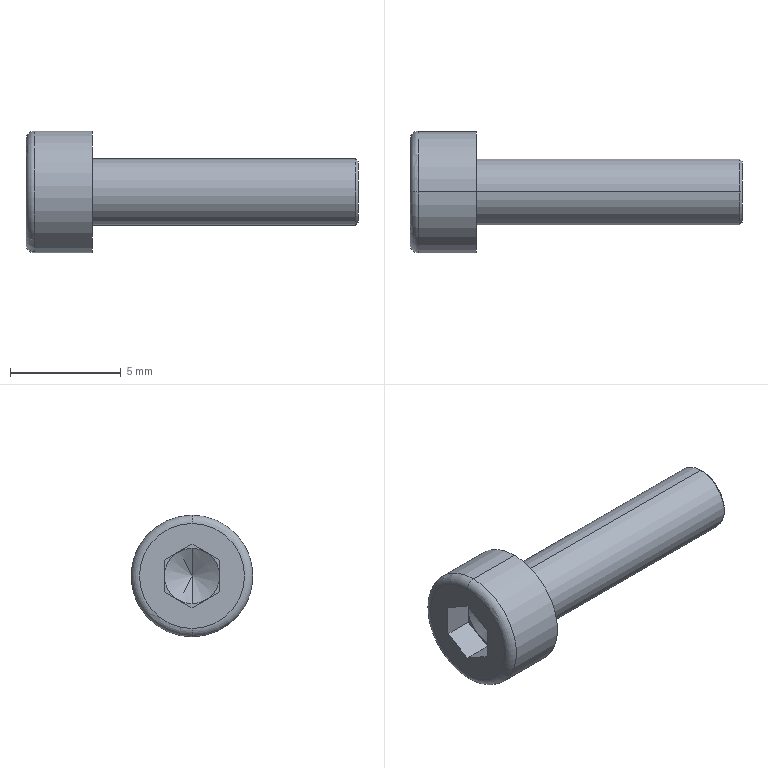Part | SolidWorks | features Fillet 2, RevCut 2, Boss 1, Chamfer 1, Cut 1, Extrusion 1, LPattern 1 | 1 solid | 25 faces | box 15 x 5.5 x 5.5 mm | volume 147.329 mm3 | plane 15 | cone 4 | cylinder 4 | torus 2 | commonest cylinder face diameters 3 x2 5.5 x2
STEP:
#1=CARTESIAN_POINT('',(15.,0.,-1.4));
#2=VERTEX_POINT('',#1);
#3=CARTESIAN_POINT('',(15.,0.,1.4));
#4=VERTEX_POINT('',#3);
#5=CARTESIAN_POINT('',(15.,0.,0.));
#6=DIRECTION('',(1.,0.,0.));
#7=DIRECTION('',(0.,0.,-1.));
#8=AXIS2_PLACEMENT_3D('',#5,#6,#7);
#9=CIRCLE('',#8,1.4);
#10=EDGE_CURVE('',#2,#4,#9,.T.);
#11=ORIENTED_EDGE('',*,*,#10,.F.);
#12=CARTESIAN_POINT('',(14.9,0.,-1.5));
#13=VERTEX_POINT('',#12);
#14=CARTESIAN_POINT('',(15.,0.,-1.4));
#15=DIRECTION('',(-0.7071,0.,-0.7071));
#16=VECTOR('',#15,1000.);
#17=LINE('',#14,#16);
#18=EDGE_CURVE('',#2,#13,#17,.T.);
#19=ORIENTED_EDGE('',*,*,#18,.T.);
#20=CARTESIAN_POINT('',(14.9,0.,1.5));
#21=VERTEX_POINT('',#20);
#22=CARTESIAN_POINT('',(14.9,0.,0.));
#23=DIRECTION('',(-1.,0.,0.));
#24=DIRECTION('',(0.,0.,-1.));
#25=AXIS2_PLACEMENT_3D('',#22,#23,#24);
#26=CIRCLE('',#25,1.5);
#27=EDGE_CURVE('',#21,#13,#26,.T.);
#28=ORIENTED_EDGE('',*,*,#27,.F.);
#29=CARTESIAN_POINT('',(15.,0.,1.4));
#30=DIRECTION('',(-0.7071,0.,0.7071));
#31=VECTOR('',#30,1000.);
#32=LINE('',#29,#31);
#33=EDGE_CURVE('',#4,#21,#32,.T.);
#34=ORIENTED_EDGE('',*,*,#33,.F.);
#35=EDGE_LOOP('',(#11,#19,#28,#34));
#36=FACE_OUTER_BOUND('',#35,.T.);
#37=CARTESIAN_POINT('',(15.,0.,0.));
#38=DIRECTION('',(-1.,0.,0.));
#39=DIRECTION('',(0.,0.,1.));
#40=AXIS2_PLACEMENT_3D('',#37,#38,#39);
#41=CONICAL_SURFACE('',#40,1.4,0.7854);
#42=ADVANCED_FACE('',(#36),#41,.T.);
#43=CARTESIAN_POINT('',(0.,0.,2.375));
#44=VERTEX_POINT('',#43);
#45=CARTESIAN_POINT('',(0.,0.,-2.375));
#46=VERTEX_POINT('',#45);
#47=CARTESIAN_POINT('',(0.,0.,0.));
#48=DIRECTION('',(-1.,0.,0.));
#49=DIRECTION('',(0.,0.,-1.));
#50=AXIS2_PLACEMENT_3D('',#47,#48,#49);
#51=CIRCLE('',#50,2.375);
#52=EDGE_CURVE('',#44,#46,#51,.T.);
#53=ORIENTED_EDGE('',*,*,#52,.F.);
#54=CARTESIAN_POINT('',(0.375,0.,2.75));
#55=VERTEX_POINT('',#54);
#56=CARTESIAN_POINT('',(0.375,0.,2.375));
#57=DIRECTION('',(0.,1.,0.));
#58=DIRECTION('',(0.,0.,1.));
#59=AXIS2_PLACEMENT_3D('',#56,#57,#58);
#60=CIRCLE('',#59,0.375);
#61=EDGE_CURVE('',#44,#55,#60,.T.);
#62=ORIENTED_EDGE('',*,*,#61,.T.);
#63=CARTESIAN_POINT('',(0.375,0.,-2.75));
#64=VERTEX_POINT('',#63);
#65=CARTESIAN_POINT('',(0.375,0.,0.));
#66=DIRECTION('',(1.,0.,0.));
#67=DIRECTION('',(0.,0.,-1.));
#68=AXIS2_PLACEMENT_3D('',#65,#66,#67);
#69=CIRCLE('',#68,2.75);
#70=EDGE_CURVE('',#64,#55,#69,.T.);
#71=ORIENTED_EDGE('',*,*,#70,.F.);
#72=CARTESIAN_POINT('',(0.375,0.,-2.375));
#73=DIRECTION('',(0.,-1.,0.));
#74=DIRECTION('',(0.,0.,-1.));
#75=AXIS2_PLACEMENT_3D('',#72,#73,#74);
#76=CIRCLE('',#75,0.375);
#77=EDGE_CURVE('',#46,#64,#76,.T.);
#78=ORIENTED_EDGE('',*,*,#77,.F.);
#79=EDGE_LOOP('',(#53,#62,#71,#78));
#80=FACE_OUTER_BOUND('',#79,.T.);
#81=CARTESIAN_POINT('',(0.375,0.,0.));
#82=DIRECTION('',(1.,0.,0.));
#83=DIRECTION('',(0.,0.,-1.));
#84=AXIS2_PLACEMENT_3D('',#81,#82,#83);
#85=TOROIDAL_SURFACE('',#84,2.375,0.375);
#86=ADVANCED_FACE('',(#80),#85,.T.);
#87=CARTESIAN_POINT('',(2.022,0.,0.));
#88=VERTEX_POINT('',#87);
#89=CARTESIAN_POINT('',(1.3,0.,1.25));
#90=VERTEX_POINT('',#89);
#91=CARTESIAN_POINT('',(1.3,0.,1.25));
#92=DIRECTION('',(-0.5,0.,0.866));
#93=VECTOR('',#92,1000.);
#94=LINE('',#91,#93);
#95=EDGE_CURVE('',#88,#90,#94,.T.);
#96=ORIENTED_EDGE('',*,*,#95,.F.);
#97=CARTESIAN_POINT('',(1.3,0.,-1.25));
#98=VERTEX_POINT('',#97);
#99=CARTESIAN_POINT('',(1.3,0.,-1.25));
#100=DIRECTION('',(-0.5,0.,-0.866));
#101=VECTOR('',#100,1000.);
#102=LINE('',#99,#101);
#103=EDGE_CURVE('',#88,#98,#102,.T.);
#104=ORIENTED_EDGE('',*,*,#103,.T.);
#105=CARTESIAN_POINT('',(1.3,-0.625,-1.083));
#106=VERTEX_POINT('',#105);
#107=CARTESIAN_POINT('',(1.3,0.,0.));
#108=DIRECTION('',(1.,0.,0.));
#109=DIRECTION('',(0.,0.,1.));
#110=AXIS2_PLACEMENT_3D('',#107,#108,#109);
#111=CIRCLE('',#110,1.25);
#112=EDGE_CURVE('',#106,#98,#111,.T.);
#113=ORIENTED_EDGE('',*,*,#112,.F.);
#114=CARTESIAN_POINT('',(1.3,-1.25,0.));
#115=VERTEX_POINT('',#114);
#116=CARTESIAN_POINT('',(1.3,0.,0.));
#117=DIRECTION('',(1.,0.,0.));
#118=DIRECTION('',(0.,0.,1.));
#119=AXIS2_PLACEMENT_3D('',#116,#117,#118);
#120=CIRCLE('',#119,1.25);
#121=EDGE_CURVE('',#115,#106,#120,.T.);
#122=ORIENTED_EDGE('',*,*,#121,.F.);
#123=CARTESIAN_POINT('',(1.3,-0.625,1.083));
#124=VERTEX_POINT('',#123);
#125=CARTESIAN_POINT('',(1.3,0.,0.));
#126=DIRECTION('',(1.,0.,0.));
#127=DIRECTION('',(0.,0.,1.));
#128=AXIS2_PLACEMENT_3D('',#125,#126,#127);
#129=CIRCLE('',#128,1.25);
#130=EDGE_CURVE('',#124,#115,#129,.T.);
#131=ORIENTED_EDGE('',*,*,#130,.F.);
#132=CARTESIAN_POINT('',(1.3,0.,0.));
#133=DIRECTION('',(1.,0.,0.));
#134=DIRECTION('',(0.,0.,1.));
#135=AXIS2_PLACEMENT_3D('',#132,#133,#134);
#136=CIRCLE('',#135,1.25);
#137=EDGE_CURVE('',#90,#124,#136,.T.);
#138=ORIENTED_EDGE('',*,*,#137,.F.);
#139=EDGE_LOOP('',(#96,#104,#113,#122,#131,#138));
#140=FACE_OUTER_BOUND('',#139,.T.);
#141=CARTESIAN_POINT('',(1.3,0.,0.));
#142=DIRECTION('',(-1.,0.,0.));
#143=DIRECTION('',(0.,0.,1.));
#144=AXIS2_PLACEMENT_3D('',#141,#142,#143);
#145=CONICAL_SURFACE('',#144,1.25,1.047);
#146=ADVANCED_FACE('',(#140),#145,.F.);
#147=ORIENTED_EDGE('',*,*,#27,.T.);
#148=CARTESIAN_POINT('',(3.,0.,-1.5));
#149=VERTEX_POINT('',#148);
#150=CARTESIAN_POINT('',(15.,0.,-1.5));
#151=DIRECTION('',(-1.,0.,0.));
#152=VECTOR('',#151,1000.);
#153=LINE('',#150,#152);
#154=EDGE_CURVE('',#13,#149,#153,.T.);
#155=ORIENTED_EDGE('',*,*,#154,.T.);
#156=CARTESIAN_POINT('',(3.,0.,1.5));
#157=VERTEX_POINT('',#156);
#158=CARTESIAN_POINT('',(3.,0.,0.));
#159=DIRECTION('',(1.,0.,0.));
#160=DIRECTION('',(0.,0.,-1.));
#161=AXIS2_PLACEMENT_3D('',#158,#159,#160);
#162=CIRCLE('',#161,1.5);
#163=EDGE_CURVE('',#149,#157,#162,.T.);
#164=ORIENTED_EDGE('',*,*,#163,.T.);
#165=CARTESIAN_POINT('',(15.,0.,1.5));
#166=DIRECTION('',(-1.,0.,0.));
#167=VECTOR('',#166,1000.);
#168=LINE('',#165,#167);
#169=EDGE_CURVE('',#21,#157,#168,.T.);
#170=ORIENTED_EDGE('',*,*,#169,.F.);
#171=EDGE_LOOP('',(#147,#155,#164,#170));
#172=FACE_OUTER_BOUND('',#171,.T.);
#173=CARTESIAN_POINT('',(15.,0.,0.));
#174=DIRECTION('',(-1.,0.,0.));
#175=DIRECTION('',(0.,0.,1.));
#176=AXIS2_PLACEMENT_3D('',#173,#174,#175);
#177=CYLINDRICAL_SURFACE('',#176,1.5);
#178=ADVANCED_FACE('',(#172),#177,.T.);
#179=CARTESIAN_POINT('',(3.,0.,-2.75));
#180=VERTEX_POINT('',#179);
#181=CARTESIAN_POINT('',(3.,0.,2.75));
#182=VERTEX_POINT('',#181);
#183=CARTESIAN_POINT('',(3.,0.,0.));
#184=DIRECTION('',(1.,0.,0.));
#185=DIRECTION('',(0.,0.,-1.));
#186=AXIS2_PLACEMENT_3D('',#183,#184,#185);
#187=CIRCLE('',#186,2.75);
#188=EDGE_CURVE('',#180,#182,#187,.T.);
#189=ORIENTED_EDGE('',*,*,#188,.F.);
#190=CARTESIAN_POINT('',(3.,0.,-2.75));
#191=DIRECTION('',(-1.,0.,0.));
#192=VECTOR('',#191,1000.);
#193=LINE('',#190,#192);
#194=EDGE_CURVE('',#180,#64,#193,.T.);
#195=ORIENTED_EDGE('',*,*,#194,.T.);
#196=ORIENTED_EDGE('',*,*,#70,.T.);
#197=CARTESIAN_POINT('',(3.,0.,2.75));
#198=DIRECTION('',(-1.,0.,0.));
#199=VECTOR('',#198,1000.);
#200=LINE('',#197,#199);
#201=EDGE_CURVE('',#182,#55,#200,.T.);
#202=ORIENTED_EDGE('',*,*,#201,.F.);
#203=EDGE_LOOP('',(#189,#195,#196,#202));
#204=FACE_OUTER_BOUND('',#203,.T.);
#205=CARTESIAN_POINT('',(3.,0.,0.));
#206=DIRECTION('',(-1.,0.,0.));
#207=DIRECTION('',(0.,0.,1.));
#208=AXIS2_PLACEMENT_3D('',#205,#206,#207);
#209=CYLINDRICAL_SURFACE('',#208,2.75);
#210=ADVANCED_FACE('',(#204),#209,.T.);
#211=CARTESIAN_POINT('',(1.3,-1.25,0.7217));
#212=VERTEX_POINT('',#211);
#213=CARTESIAN_POINT('',(1.3,0.,1.443));
#214=DIRECTION('',(0.,-0.866,-0.5));
#215=VECTOR('',#214,1000.);
#216=LINE('',#213,#215);
#217=EDGE_CURVE('',#124,#212,#216,.T.);
#218=ORIENTED_EDGE('',*,*,#217,.F.);
#219=ORIENTED_EDGE('',*,*,#130,.T.);
#220=CARTESIAN_POINT('',(1.3,-1.25,0.7217));
#221=DIRECTION('',(0.,0.,-1.));
#222=VECTOR('',#221,1000.);
#223=LINE('',#220,#222);
#224=EDGE_CURVE('',#212,#115,#223,.T.);
#225=ORIENTED_EDGE('',*,*,#224,.F.);
#226=EDGE_LOOP('',(#218,#219,#225));
#227=FACE_OUTER_BOUND('',#226,.T.);
#228=CARTESIAN_POINT('',(1.3,-2.5,0.));
#229=DIRECTION('',(-1.,0.,0.));
#230=DIRECTION('',(0.,0.,1.));
#231=AXIS2_PLACEMENT_3D('',#228,#229,#230);
#232=PLANE('',#231);
#233=ADVANCED_FACE('',(#227),#232,.T.);
#234=CARTESIAN_POINT('',(1.3,-1.25,-0.7217));
#235=VERTEX_POINT('',#234);
#236=CARTESIAN_POINT('',(1.3,-1.25,0.7217));
#237=DIRECTION('',(0.,0.,-1.));
#238=VECTOR('',#237,1000.);
#239=LINE('',#236,#238);
#240=EDGE_CURVE('',#115,#235,#239,.T.);
#241=ORIENTED_EDGE('',*,*,#240,.F.);
#242=ORIENTED_EDGE('',*,*,#121,.T.);
#243=CARTESIAN_POINT('',(1.3,-1.25,-0.7217));
#244=DIRECTION('',(0.,0.866,-0.5));
#245=VECTOR('',#244,1000.);
#246=LINE('',#243,#245);
#247=EDGE_CURVE('',#235,#106,#246,.T.);
#248=ORIENTED_EDGE('',*,*,#247,.F.);
#249=EDGE_LOOP('',(#241,#242,#248));
#250=FACE_OUTER_BOUND('',#249,.T.);
#251=CARTESIAN_POINT('',(1.3,-2.5,0.));
#252=DIRECTION('',(-1.,0.,0.));
#253=DIRECTION('',(0.,0.,1.));
#254=AXIS2_PLACEMENT_3D('',#251,#252,#253);
#255=PLANE('',#254);
#256=ADVANCED_FACE('',(#250),#255,.T.);
#257=CARTESIAN_POINT('',(1.3,0.,-1.443));
#258=VERTEX_POINT('',#257);
#259=CARTESIAN_POINT('',(1.3,-1.25,-0.7217));
#260=DIRECTION('',(0.,0.866,-0.5));
#261=VECTOR('',#260,1000.);
#262=LINE('',#259,#261);
#263=EDGE_CURVE('',#106,#258,#262,.T.);
#264=ORIENTED_EDGE('',*,*,#263,.F.);
#265=ORIENTED_EDGE('',*,*,#112,.T.);
#266=CARTESIAN_POINT('',(1.3,0.625,-1.083));
#267=VERTEX_POINT('',#266);
#268=CARTESIAN_POINT('',(1.3,0.,0.));
#269=DIRECTION('',(1.,0.,0.));
#270=DIRECTION('',(0.,0.,1.));
#271=AXIS2_PLACEMENT_3D('',#268,#269,#270);
#272=CIRCLE('',#271,1.25);
#273=EDGE_CURVE('',#98,#267,#272,.T.);
#274=ORIENTED_EDGE('',*,*,#273,.T.);
#275=CARTESIAN_POINT('',(1.3,0.,-1.443));
#276=DIRECTION('',(0.,0.866,0.5));
#277=VECTOR('',#276,1000.);
#278=LINE('',#275,#277);
#279=EDGE_CURVE('',#258,#267,#278,.T.);
#280=ORIENTED_EDGE('',*,*,#279,.F.);
#281=EDGE_LOOP('',(#264,#265,#274,#280));
#282=FACE_OUTER_BOUND('',#281,.T.);
#283=CARTESIAN_POINT('',(1.3,-2.5,0.));
#284=DIRECTION('',(-1.,0.,0.));
#285=DIRECTION('',(0.,0.,1.));
#286=AXIS2_PLACEMENT_3D('',#283,#284,#285);
#287=PLANE('',#286);
#288=ADVANCED_FACE('',(#282),#287,.T.);
#289=CARTESIAN_POINT('',(1.3,1.25,-0.7217));
#290=VERTEX_POINT('',#289);
#291=CARTESIAN_POINT('',(1.3,0.,-1.443));
#292=DIRECTION('',(0.,0.866,0.5));
#293=VECTOR('',#292,1000.);
#294=LINE('',#291,#293);
#295=EDGE_CURVE('',#267,#290,#294,.T.);
#296=ORIENTED_EDGE('',*,*,#295,.F.);
#297=CARTESIAN_POINT('',(1.3,1.25,0.));
#298=VERTEX_POINT('',#297);
#299=CARTESIAN_POINT('',(1.3,0.,0.));
#300=DIRECTION('',(1.,0.,0.));
#301=DIRECTION('',(0.,0.,-1.));
#302=AXIS2_PLACEMENT_3D('',#299,#300,#301);
#303=CIRCLE('',#302,1.25);
#304=EDGE_CURVE('',#267,#298,#303,.T.);
#305=ORIENTED_EDGE('',*,*,#304,.T.);
#306=CARTESIAN_POINT('',(1.3,1.25,-0.7217));
#307=DIRECTION('',(0.,0.,1.));
#308=VECTOR('',#307,1000.);
#309=LINE('',#306,#308);
#310=EDGE_CURVE('',#290,#298,#309,.T.);
#311=ORIENTED_EDGE('',*,*,#310,.F.);
#312=EDGE_LOOP('',(#296,#305,#311));
#313=FACE_OUTER_BOUND('',#312,.T.);
#314=CARTESIAN_POINT('',(1.3,-2.5,0.));
#315=DIRECTION('',(-1.,0.,0.));
#316=DIRECTION('',(0.,0.,1.));
#317=AXIS2_PLACEMENT_3D('',#314,#315,#316);
#318=PLANE('',#317);
#319=ADVANCED_FACE('',(#313),#318,.T.);
#320=CARTESIAN_POINT('',(1.3,1.25,0.7217));
#321=VERTEX_POINT('',#320);
#322=CARTESIAN_POINT('',(1.3,1.25,-0.7217));
#323=DIRECTION('',(0.,0.,1.));
#324=VECTOR('',#323,1000.);
#325=LINE('',#322,#324);
#326=EDGE_CURVE('',#298,#321,#325,.T.);
#327=ORIENTED_EDGE('',*,*,#326,.F.);
#328=CARTESIAN_POINT('',(1.3,0.625,1.083));
#329=VERTEX_POINT('',#328);
#330=CARTESIAN_POINT('',(1.3,0.,0.));
#331=DIRECTION('',(1.,0.,0.));
#332=DIRECTION('',(0.,0.,1.));
#333=AXIS2_PLACEMENT_3D('',#330,#331,#332);
#334=CIRCLE('',#333,1.25);
#335=EDGE_CURVE('',#298,#329,#334,.T.);
#336=ORIENTED_EDGE('',*,*,#335,.T.);
#337=CARTESIAN_POINT('',(1.3,1.25,0.7217));
#338=DIRECTION('',(0.,-0.866,0.5));
#339=VECTOR('',#338,1000.);
#340=LINE('',#337,#339);
#341=EDGE_CURVE('',#321,#329,#340,.T.);
#342=ORIENTED_EDGE('',*,*,#341,.F.);
#343=EDGE_LOOP('',(#327,#336,#342));
#344=FACE_OUTER_BOUND('',#343,.T.);
#345=CARTESIAN_POINT('',(1.3,-2.5,0.));
#346=DIRECTION('',(-1.,0.,0.));
#347=DIRECTION('',(0.,0.,1.));
#348=AXIS2_PLACEMENT_3D('',#345,#346,#347);
#349=PLANE('',#348);
#350=ADVANCED_FACE('',(#344),#349,.T.);
#351=CARTESIAN_POINT('',(1.3,0.,1.443));
#352=VERTEX_POINT('',#351);
#353=CARTESIAN_POINT('',(1.3,1.25,0.7217));
#354=DIRECTION('',(0.,-0.866,0.5));
#355=VECTOR('',#354,1000.);
#356=LINE('',#353,#355);
#357=EDGE_CURVE('',#329,#352,#356,.T.);
#358=ORIENTED_EDGE('',*,*,#357,.F.);
#359=CARTESIAN_POINT('',(1.3,0.,0.));
#360=DIRECTION('',(1.,0.,0.));
#361=DIRECTION('',(0.,0.,1.));
#362=AXIS2_PLACEMENT_3D('',#359,#360,#361);
#363=CIRCLE('',#362,1.25);
#364=EDGE_CURVE('',#329,#90,#363,.T.);
#365=ORIENTED_EDGE('',*,*,#364,.T.);
#366=ORIENTED_EDGE('',*,*,#137,.T.);
#367=CARTESIAN_POINT('',(1.3,0.,1.443));
#368=DIRECTION('',(0.,-0.866,-0.5));
#369=VECTOR('',#368,1000.);
#370=LINE('',#367,#369);
#371=EDGE_CURVE('',#352,#124,#370,.T.);
#372=ORIENTED_EDGE('',*,*,#371,.F.);
#373=EDGE_LOOP('',(#358,#365,#366,#372));
#374=FACE_OUTER_BOUND('',#373,.T.);
#375=CARTESIAN_POINT('',(1.3,-2.5,0.));
#376=DIRECTION('',(-1.,0.,0.));
#377=DIRECTION('',(0.,0.,1.));
#378=AXIS2_PLACEMENT_3D('',#375,#376,#377);
#379=PLANE('',#378);
#380=ADVANCED_FACE('',(#374),#379,.T.);
#381=CARTESIAN_POINT('',(0.,0.,0.));
#382=DIRECTION('',(-1.,0.,0.));
#383=DIRECTION('',(0.,0.,-1.));
#384=AXIS2_PLACEMENT_3D('',#381,#382,#383);
#385=CIRCLE('',#384,2.375);
#386=EDGE_CURVE('',#46,#44,#385,.T.);
#387=ORIENTED_EDGE('',*,*,#386,.T.);
#388=ORIENTED_EDGE('',*,*,#52,.T.);
#389=EDGE_LOOP('',(#387,#388));
#390=FACE_OUTER_BOUND('',#389,.T.);
#391=CARTESIAN_POINT('',(0.,-1.25,-0.7217));
#392=VERTEX_POINT('',#391);
#393=CARTESIAN_POINT('',(0.,0.,-1.443));
#394=VERTEX_POINT('',#393);
#395=CARTESIAN_POINT('',(0.,-1.25,-0.7217));
#396=DIRECTION('',(0.,0.866,-0.5));
#397=VECTOR('',#396,1000.);
#398=LINE('',#395,#397);
#399=EDGE_CURVE('',#392,#394,#398,.T.);
#400=ORIENTED_EDGE('',*,*,#399,.T.);
#401=CARTESIAN_POINT('',(0.,1.25,-0.7217));
#402=VERTEX_POINT('',#401);
#403=CARTESIAN_POINT('',(0.,0.,-1.443));
#404=DIRECTION('',(0.,0.866,0.5));
#405=VECTOR('',#404,1000.);
#406=LINE('',#403,#405);
#407=EDGE_CURVE('',#394,#402,#406,.T.);
#408=ORIENTED_EDGE('',*,*,#407,.T.);
#409=CARTESIAN_POINT('',(0.,1.25,0.7217));
#410=VERTEX_POINT('',#409);
#411=CARTESIAN_POINT('',(0.,1.25,-0.7217));
#412=DIRECTION('',(0.,0.,1.));
#413=VECTOR('',#412,1000.);
#414=LINE('',#411,#413);
#415=EDGE_CURVE('',#402,#410,#414,.T.);
#416=ORIENTED_EDGE('',*,*,#415,.T.);
#417=CARTESIAN_POINT('',(0.,0.,1.443));
#418=VERTEX_POINT('',#417);
#419=CARTESIAN_POINT('',(0.,1.25,0.7217));
#420=DIRECTION('',(0.,-0.866,0.5));
#421=VECTOR('',#420,1000.);
#422=LINE('',#419,#421);
#423=EDGE_CURVE('',#410,#418,#422,.T.);
#424=ORIENTED_EDGE('',*,*,#423,.T.);
#425=CARTESIAN_POINT('',(0.,-1.25,0.7217));
#426=VERTEX_POINT('',#425);
#427=CARTESIAN_POINT('',(0.,0.,1.443));
#428=DIRECTION('',(0.,-0.866,-0.5));
#429=VECTOR('',#428,1000.);
#430=LINE('',#427,#429);
#431=EDGE_CURVE('',#418,#426,#430,.T.);
#432=ORIENTED_EDGE('',*,*,#431,.T.);
#433=CARTESIAN_POINT('',(0.,-1.25,0.7217));
#434=DIRECTION('',(0.,0.,-1.));
#435=VECTOR('',#434,1000.);
#436=LINE('',#433,#435);
#437=EDGE_CURVE('',#426,#392,#436,.T.);
#438=ORIENTED_EDGE('',*,*,#437,.T.);
#439=EDGE_LOOP('',(#400,#408,#416,#424,#432,#438));
#440=FACE_BOUND('',#439,.T.);
#441=CARTESIAN_POINT('',(0.,0.,0.));
#442=DIRECTION('',(1.,0.,0.));
#443=DIRECTION('',(0.,0.,-1.));
#444=AXIS2_PLACEMENT_3D('',#441,#442,#443);
#445=PLANE('',#444);
#446=ADVANCED_FACE('',(#390,#440),#445,.F.);
#447=CARTESIAN_POINT('',(3.,0.,0.));
#448=DIRECTION('',(1.,0.,0.));
#449=DIRECTION('',(0.,0.,-1.));
#450=AXIS2_PLACEMENT_3D('',#447,#448,#449);
#451=CIRCLE('',#450,2.75);
#452=EDGE_CURVE('',#182,#180,#451,.T.);
#453=ORIENTED_EDGE('',*,*,#452,.T.);
#454=ORIENTED_EDGE('',*,*,#188,.T.);
#455=EDGE_LOOP('',(#453,#454));
#456=FACE_OUTER_BOUND('',#455,.T.);
#457=CARTESIAN_POINT('',(3.,0.,0.));
#458=DIRECTION('',(1.,0.,0.));
#459=DIRECTION('',(0.,0.,-1.));
#460=AXIS2_PLACEMENT_3D('',#457,#458,#459);
#461=CIRCLE('',#460,1.5);
#462=EDGE_CURVE('',#157,#149,#461,.T.);
#463=ORIENTED_EDGE('',*,*,#462,.F.);
#464=ORIENTED_EDGE('',*,*,#163,.F.);
#465=EDGE_LOOP('',(#463,#464));
#466=FACE_BOUND('',#465,.T.);
#467=CARTESIAN_POINT('',(3.,0.,0.));
#468=DIRECTION('',(1.,0.,0.));
#469=DIRECTION('',(0.,0.,-1.));
#470=AXIS2_PLACEMENT_3D('',#467,#468,#469);
#471=PLANE('',#470);
#472=ADVANCED_FACE('',(#456,#466),#471,.T.);
#473=ORIENTED_EDGE('',*,*,#194,.F.);
#474=ORIENTED_EDGE('',*,*,#452,.F.);
#475=ORIENTED_EDGE('',*,*,#201,.T.);
#476=CARTESIAN_POINT('',(0.375,0.,0.));
#477=DIRECTION('',(1.,0.,0.));
#478=DIRECTION('',(0.,0.,-1.));
#479=AXIS2_PLACEMENT_3D('',#476,#477,#478);
#480=CIRCLE('',#479,2.75);
#481=EDGE_CURVE('',#55,#64,#480,.T.);
#482=ORIENTED_EDGE('',*,*,#481,.T.);
#483=EDGE_LOOP('',(#473,#474,#475,#482));
#484=FACE_OUTER_BOUND('',#483,.T.);
#485=CARTESIAN_POINT('',(3.,0.,0.));
#486=DIRECTION('',(-1.,0.,0.));
#487=DIRECTION('',(0.,0.,1.));
#488=AXIS2_PLACEMENT_3D('',#485,#486,#487);
#489=CYLINDRICAL_SURFACE('',#488,2.75);
#490=ADVANCED_FACE('',(#484),#489,.T.);
#491=ORIENTED_EDGE('',*,*,#154,.F.);
#492=CARTESIAN_POINT('',(14.9,0.,0.));
#493=DIRECTION('',(-1.,0.,0.));
#494=DIRECTION('',(0.,0.,-1.));
#495=AXIS2_PLACEMENT_3D('',#492,#493,#494);
#496=CIRCLE('',#495,1.5);
#497=EDGE_CURVE('',#13,#21,#496,.T.);
#498=ORIENTED_EDGE('',*,*,#497,.T.);
#499=ORIENTED_EDGE('',*,*,#169,.T.);
#500=ORIENTED_EDGE('',*,*,#462,.T.);
#501=EDGE_LOOP('',(#491,#498,#499,#500));
#502=FACE_OUTER_BOUND('',#501,.T.);
#503=CARTESIAN_POINT('',(15.,0.,0.));
#504=DIRECTION('',(-1.,0.,0.));
#505=DIRECTION('',(0.,0.,1.));
#506=AXIS2_PLACEMENT_3D('',#503,#504,#505);
#507=CYLINDRICAL_SURFACE('',#506,1.5);
#508=ADVANCED_FACE('',(#502),#507,.T.);
#509=CARTESIAN_POINT('',(15.,0.,0.));
#510=DIRECTION('',(1.,0.,0.));
#511=DIRECTION('',(0.,0.,-1.));
#512=AXIS2_PLACEMENT_3D('',#509,#510,#511);
#513=CIRCLE('',#512,1.4);
#514=EDGE_CURVE('',#4,#2,#513,.T.);
#515=ORIENTED_EDGE('',*,*,#514,.T.);
#516=ORIENTED_EDGE('',*,*,#10,.T.);
#517=EDGE_LOOP('',(#515,#516));
#518=FACE_OUTER_BOUND('',#517,.T.);
#519=CARTESIAN_POINT('',(15.,0.,0.));
#520=DIRECTION('',(1.,0.,0.));
#521=DIRECTION('',(0.,0.,-1.));
#522=AXIS2_PLACEMENT_3D('',#519,#520,#521);
#523=PLANE('',#522);
#524=ADVANCED_FACE('',(#518),#523,.T.);
#525=ORIENTED_EDGE('',*,*,#399,.F.);
#526=CARTESIAN_POINT('',(1.3,-1.25,-0.7217));
#527=DIRECTION('',(-1.,0.,0.));
#528=VECTOR('',#527,1000.);
#529=LINE('',#526,#528);
#530=EDGE_CURVE('',#235,#392,#529,.T.);
#531=ORIENTED_EDGE('',*,*,#530,.F.);
#532=ORIENTED_EDGE('',*,*,#247,.T.);
#533=ORIENTED_EDGE('',*,*,#263,.T.);
#534=CARTESIAN_POINT('',(1.3,0.,-1.443));
#535=DIRECTION('',(-1.,0.,0.));
#536=VECTOR('',#535,1000.);
#537=LINE('',#534,#536);
#538=EDGE_CURVE('',#258,#394,#537,.T.);
#539=ORIENTED_EDGE('',*,*,#538,.T.);
#540=EDGE_LOOP('',(#525,#531,#532,#533,#539));
#541=FACE_OUTER_BOUND('',#540,.T.);
#542=CARTESIAN_POINT('',(1.3,-1.25,-0.7217));
#543=DIRECTION('',(0.,0.5,0.866));
#544=DIRECTION('',(0.,-0.866,0.5));
#545=AXIS2_PLACEMENT_3D('',#542,#543,#544);
#546=PLANE('',#545);
#547=ADVANCED_FACE('',(#541),#546,.T.);
#548=ORIENTED_EDGE('',*,*,#407,.F.);
#549=ORIENTED_EDGE('',*,*,#538,.F.);
#550=ORIENTED_EDGE('',*,*,#279,.T.);
#551=ORIENTED_EDGE('',*,*,#295,.T.);
#552=CARTESIAN_POINT('',(1.3,1.25,-0.7217));
#553=DIRECTION('',(-1.,0.,0.));
#554=VECTOR('',#553,1000.);
#555=LINE('',#552,#554);
#556=EDGE_CURVE('',#290,#402,#555,.T.);
#557=ORIENTED_EDGE('',*,*,#556,.T.);
#558=EDGE_LOOP('',(#548,#549,#550,#551,#557));
#559=FACE_OUTER_BOUND('',#558,.T.);
#560=CARTESIAN_POINT('',(1.3,0.,-1.443));
#561=DIRECTION('',(0.,-0.5,0.866));
#562=DIRECTION('',(0.,-0.866,-0.5));
#563=AXIS2_PLACEMENT_3D('',#560,#561,#562);
#564=PLANE('',#563);
#565=ADVANCED_FACE('',(#559),#564,.T.);
#566=ORIENTED_EDGE('',*,*,#415,.F.);
#567=ORIENTED_EDGE('',*,*,#556,.F.);
#568=ORIENTED_EDGE('',*,*,#310,.T.);
#569=ORIENTED_EDGE('',*,*,#326,.T.);
#570=CARTESIAN_POINT('',(1.3,1.25,0.7217));
#571=DIRECTION('',(-1.,0.,0.));
#572=VECTOR('',#571,1000.);
#573=LINE('',#570,#572);
#574=EDGE_CURVE('',#321,#410,#573,.T.);
#575=ORIENTED_EDGE('',*,*,#574,.T.);
#576=EDGE_LOOP('',(#566,#567,#568,#569,#575));
#577=FACE_OUTER_BOUND('',#576,.T.);
#578=CARTESIAN_POINT('',(1.3,1.25,-0.7217));
#579=DIRECTION('',(0.,-1.,0.));
#580=DIRECTION('',(0.,0.,-1.));
#581=AXIS2_PLACEMENT_3D('',#578,#579,#580);
#582=PLANE('',#581);
#583=ADVANCED_FACE('',(#577),#582,.T.);
#584=ORIENTED_EDGE('',*,*,#423,.F.);
#585=ORIENTED_EDGE('',*,*,#574,.F.);
#586=ORIENTED_EDGE('',*,*,#341,.T.);
#587=ORIENTED_EDGE('',*,*,#357,.T.);
#588=CARTESIAN_POINT('',(1.3,0.,1.443));
#589=DIRECTION('',(-1.,0.,0.));
#590=VECTOR('',#589,1000.);
#591=LINE('',#588,#590);
#592=EDGE_CURVE('',#352,#418,#591,.T.);
#593=ORIENTED_EDGE('',*,*,#592,.T.);
#594=EDGE_LOOP('',(#584,#585,#586,#587,#593));
#595=FACE_OUTER_BOUND('',#594,.T.);
#596=CARTESIAN_POINT('',(1.3,1.25,0.7217));
#597=DIRECTION('',(0.,-0.5,-0.866));
#598=DIRECTION('',(0.,0.866,-0.5));
#599=AXIS2_PLACEMENT_3D('',#596,#597,#598);
#600=PLANE('',#599);
#601=ADVANCED_FACE('',(#595),#600,.T.);
#602=ORIENTED_EDGE('',*,*,#431,.F.);
#603=ORIENTED_EDGE('',*,*,#592,.F.);
#604=ORIENTED_EDGE('',*,*,#371,.T.);
#605=ORIENTED_EDGE('',*,*,#217,.T.);
#606=CARTESIAN_POINT('',(1.3,-1.25,0.7217));
#607=DIRECTION('',(-1.,0.,0.));
#608=VECTOR('',#607,1000.);
#609=LINE('',#606,#608);
#610=EDGE_CURVE('',#212,#426,#609,.T.);
#611=ORIENTED_EDGE('',*,*,#610,.T.);
#612=EDGE_LOOP('',(#602,#603,#604,#605,#611));
#613=FACE_OUTER_BOUND('',#612,.T.);
#614=CARTESIAN_POINT('',(1.3,0.,1.443));
#615=DIRECTION('',(0.,0.5,-0.866));
#616=DIRECTION('',(0.,0.866,0.5));
#617=AXIS2_PLACEMENT_3D('',#614,#615,#616);
#618=PLANE('',#617);
#619=ADVANCED_FACE('',(#613),#618,.T.);
#620=ORIENTED_EDGE('',*,*,#437,.F.);
#621=ORIENTED_EDGE('',*,*,#610,.F.);
#622=ORIENTED_EDGE('',*,*,#224,.T.);
#623=ORIENTED_EDGE('',*,*,#240,.T.);
#624=ORIENTED_EDGE('',*,*,#530,.T.);
#625=EDGE_LOOP('',(#620,#621,#622,#623,#624));
#626=FACE_OUTER_BOUND('',#625,.T.);
#627=CARTESIAN_POINT('',(1.3,-1.25,0.7217));
#628=DIRECTION('',(0.,1.,0.));
#629=DIRECTION('',(0.,0.,1.));
#630=AXIS2_PLACEMENT_3D('',#627,#628,#629);
#631=PLANE('',#630);
#632=ADVANCED_FACE('',(#626),#631,.T.);
#633=ORIENTED_EDGE('',*,*,#103,.F.);
#634=ORIENTED_EDGE('',*,*,#95,.T.);
#635=ORIENTED_EDGE('',*,*,#364,.F.);
#636=ORIENTED_EDGE('',*,*,#335,.F.);
#637=ORIENTED_EDGE('',*,*,#304,.F.);
#638=ORIENTED_EDGE('',*,*,#273,.F.);
#639=EDGE_LOOP('',(#633,#634,#635,#636,#637,#638));
#640=FACE_OUTER_BOUND('',#639,.T.);
#641=CARTESIAN_POINT('',(1.3,0.,0.));
#642=DIRECTION('',(-1.,0.,0.));
#643=DIRECTION('',(0.,0.,1.));
#644=AXIS2_PLACEMENT_3D('',#641,#642,#643);
#645=CONICAL_SURFACE('',#644,1.25,1.047);
#646=ADVANCED_FACE('',(#640),#645,.F.);
#647=ORIENTED_EDGE('',*,*,#61,.F.);
#648=ORIENTED_EDGE('',*,*,#386,.F.);
#649=ORIENTED_EDGE('',*,*,#77,.T.);
#650=ORIENTED_EDGE('',*,*,#481,.F.);
#651=EDGE_LOOP('',(#647,#648,#649,#650));
#652=FACE_OUTER_BOUND('',#651,.T.);
#653=CARTESIAN_POINT('',(0.375,0.,0.));
#654=DIRECTION('',(1.,0.,0.));
#655=DIRECTION('',(0.,0.,-1.));
#656=AXIS2_PLACEMENT_3D('',#653,#654,#655);
#657=TOROIDAL_SURFACE('',#656,2.375,0.375);
#658=ADVANCED_FACE('',(#652),#657,.T.);
#659=ORIENTED_EDGE('',*,*,#18,.F.);
#660=ORIENTED_EDGE('',*,*,#514,.F.);
#661=ORIENTED_EDGE('',*,*,#33,.T.);
#662=ORIENTED_EDGE('',*,*,#497,.F.);
#663=EDGE_LOOP('',(#659,#660,#661,#662));
#664=FACE_OUTER_BOUND('',#663,.T.);
#665=CARTESIAN_POINT('',(15.,0.,0.));
#666=DIRECTION('',(-1.,0.,0.));
#667=DIRECTION('',(0.,0.,1.));
#668=AXIS2_PLACEMENT_3D('',#665,#666,#667);
#669=CONICAL_SURFACE('',#668,1.4,0.7854);
#670=ADVANCED_FACE('',(#664),#669,.T.);
#671=CLOSED_SHELL('',(#42,#86,#146,#178,#210,#233,#256,#288,#319,#350,#380,#446,#472,#490,#508,#524,#547,#565,#583,#601,#619,#632,#646,#658,#670));
#672=MANIFOLD_SOLID_BREP('',#671);
#673=CARTESIAN_POINT('',(0.,0.,0.));
#674=DIRECTION('',(0.,0.,1.));
#675=DIRECTION('',(1.,0.,0.));
#676=AXIS2_PLACEMENT_3D('',#673,#674,#675);
#677=(LENGTH_UNIT()NAMED_UNIT(*)SI_UNIT(.MILLI.,.METRE.));
#678=UNCERTAINTY_MEASURE_WITH_UNIT(LENGTH_MEASURE(0.00001),#677,'','');
#679=(NAMED_UNIT(*)PLANE_ANGLE_UNIT()SI_UNIT($,.RADIAN.));
#680=(NAMED_UNIT(*)SI_UNIT($,.STERADIAN.)SOLID_ANGLE_UNIT());
#681=(GEOMETRIC_REPRESENTATION_CONTEXT(3)GLOBAL_UNCERTAINTY_ASSIGNED_CONTEXT((#678))GLOBAL_UNIT_ASSIGNED_CONTEXT((#677,#679,#680))REPRESENTATION_CONTEXT('',''));
#682=ADVANCED_BREP_SHAPE_REPRESENTATION('',(#672,#676),#681);